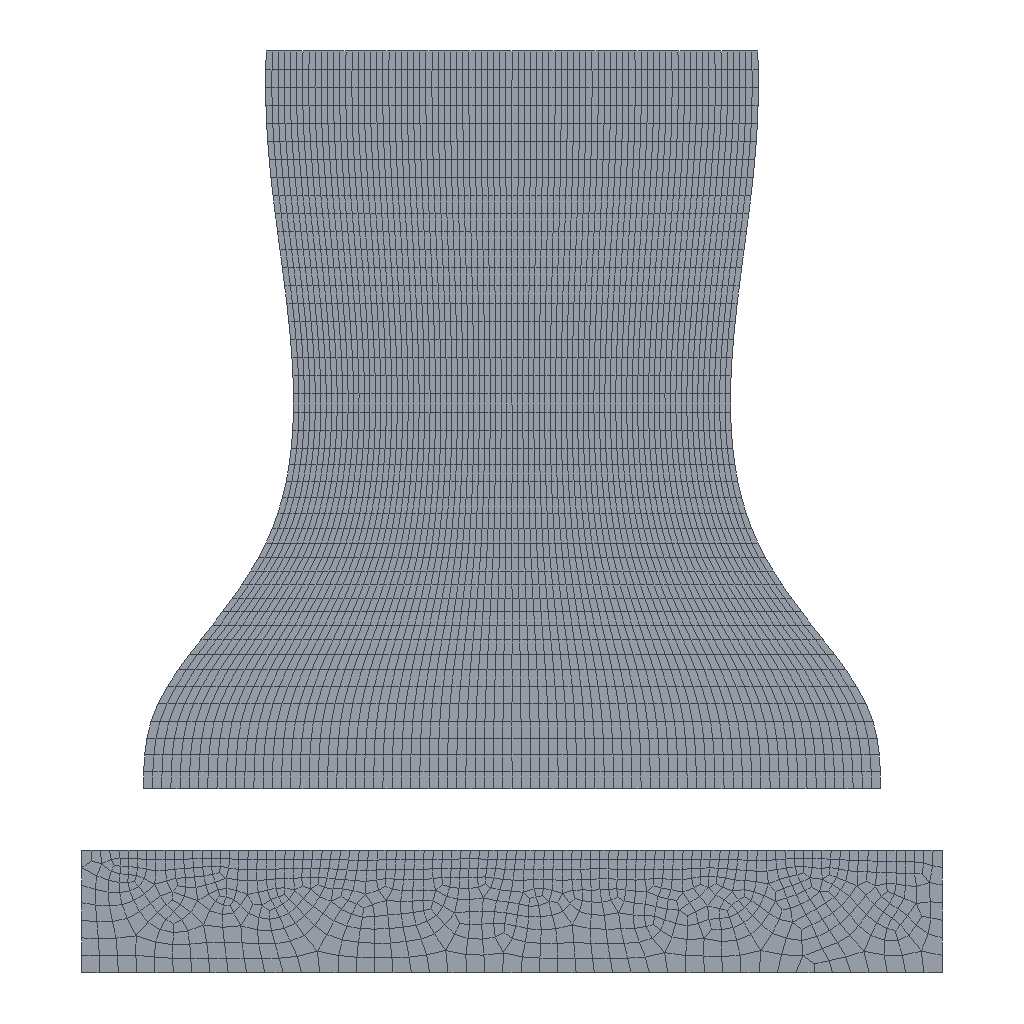Simulation study | abaqus
Set-up summary:
category,name,step,type,value,unit,region
solver,abaqus
solver,version,,,Abaqus/Standard 2020
units,not stated in the deck,,not stated
analysis,deck,,static,static
load_step,Step-1,Step-1,static
load_step,Step-3,Step-3,static
load_step,requested,,,2
mesh,nodes,,,4490
mesh,elements,,,4287
element_type,CPS4R,,plane,4287
load,load commands in deck,,count,2
bc,support commands in deck,,count,5
material,MIRROR,,in results
material,PDMS,,in results
material,SILICONRUBBER,,in results
material,TPU,,in results
material,TPU-COPY,,in results
material,TPU-COPY2,,in results
material,TPU-COPY3,,in results
material,TPU-COPY4,,in results
material,TPU-COPY5,,in results
check,setup vs results,,match,"per instance, exact: element labels, types and connectivity; labels of the nodes the elements use; coordinates of those nodes at SINGLE_PRECISION in 2 of 2 instance(s)"
Abaqus input file, long lists of numbers shortened:
*Heading
** Job name: Job-2 Model name: Model-1-Copy
** Generated by: Abaqus/CAE 2020
*Preprint, echo=NO, model=NO, history=NO, contact=NO
**
** PARTS
**
*Part, name=Mirror
*Node
      1,   137.021,           0.
      2,   131.064,           0.
** (843 more lines like these left out)
*Element, type=CPS4R
  1,  33,  31, 494,  72
  2,  72, 494, 455,  73
** (765 more lines like these left out)
*Nset, nset=_PickedSet3, internal, generate
   1,  845,    1
*Elset, elset=_PickedSet3, internal, generate
   1,  767,    1
*Elset, elset=_Surf-Mirror_S2, internal
  13,  19,  26,  33,  46,  60,  66,  72,  78,  84,  91,  95, 109, 115, 121, 127
 134, 141, 148, 154, 160, 164, 177, 183, 189, 195, 283, 344, 347, 349, 351, 353
** (2 more lines like these left out)
*Elset, elset=_Surf-Mirror_S4, internal
  40,  53, 102, 171, 284, 285, 287, 289, 290, 292, 293, 295, 296, 297, 299, 301
 303, 305, 307, 309, 310, 311, 313, 315, 317, 319, 321, 323, 325, 327, 329, 331
** (1 more lines like these left out)
*Elset, elset=_Surf-Mirror_S1, internal
 200, 383
*Elset, elset=_Surf-Mirror_S3, internal
 341,
*Surface, type=ELEMENT, name=Surf-Mirror
_Surf-Mirror_S2, S2
_Surf-Mirror_S4, S4
_Surf-Mirror_S1, S1
_Surf-Mirror_S3, S3
** Section: Section-mirror
*Solid Section, elset=_PickedSet3, material=Mirror
,
*End Part
**
*Part, name=mushroom
*Node
      1,  -35.915,   15.373
      2,   35.915,   15.373
** (3643 more lines like these left out)
*Element, type=CPS4R
   1,    1,   17,  723,  216
   2,   17,   18,  724,  723
** (3518 more lines like these left out)
*Nset, nset=FORCE
 3,
*Nset, nset=BOTTOM
  11,  12, 469, 470, 471, 472, 473, 474, 475, 476, 477, 478, 479, 480, 481, 482
 483, 484, 485, 486, 487, 488, 489, 490, 491, 492, 493, 494, 495, 496, 497, 498
** (4 more lines like these left out)
*Elset, elset=BOTTOM, generate
 2641,  2720,     1
*Nset, nset=Set-16
    1,    2,    3,    4,   17,   18,   19,   20,   21,   22,   23,   24,   25,   26,   27,   28
   29,   30,   31,   32,   33,   34,   35,   36,   37,   38,   39,   40,   41,   42,   43,   44
** (115 more lines like these left out)
*Elset, elset=Set-16, generate
    1,  1760,     1
*Nset, nset=Set-17
    9,   10,   11,   12,  387,  388,  389,  390,  391,  392,  393,  394,  395,  396,  397,  398
  399,  400,  401,  402,  403,  404,  405,  406,  407,  408,  409,  410,  411,  412,  413,  414
** (24 more lines like these left out)
*Elset, elset=Set-17, generate
 2401,  2720,     1
*Nset, nset=Set-18
    9,   10,   15,   16,  387,  388,  389,  390,  391,  392,  393,  394,  395,  396,  397,  398
  399,  400,  401,  402,  403,  404,  405,  406,  407,  408,  409,  410,  411,  412,  413,  414
** (19 more lines like these left out)
*Elset, elset=Set-18, generate
 3041,  3280,     1
*Nset, nset=Set-19
   13,   14,   15,   16,  554,  555,  556,  557,  558,  559,  560,  561,  562,  563,  564,  565
  566,  567,  568,  569,  570,  571,  572,  573,  574,  575,  576,  577,  578,  579,  580,  581
** (19 more lines like these left out)
*Elset, elset=Set-19, generate
 3281,  3520,     1
*Nset, nset=Set-20
    7,    8,   13,   14,  302,  303,  304,  305,  306,  307,  308,  309,  310,  311,  312,  313
  314,  315,  316,  317,  318,  319,  320,  321,  322,  323,  324,  325,  326,  327,  328,  329
** (24 more lines like these left out)
*Elset, elset=Set-20, generate
 2721,  3040,     1
*Nset, nset=Set-21
    5,    6,    7,    8,  220,  221,  222,  223,  224,  225,  226,  227,  228,  229,  230,  231
  232,  233,  234,  235,  236,  237,  238,  239,  240,  241,  242,  243,  244,  245,  246,  247
** (24 more lines like these left out)
*Elset, elset=Set-21, generate
 2081,  2400,     1
*Nset, nset=Set-22
    1,    2,    5,    6,   17,   18,   19,   20,   21,   22,   23,   24,   25,   26,   27,   28
   29,   30,   31,   32,   33,   34,   35,   36,   37,   38,   39,   40,   41,   42,   43,   44
** (24 more lines like these left out)
*Elset, elset=Set-22, generate
 1761,  2080,     1
*Elset, elset=_Surf-BOTTOM_S3, internal, generate
 2641,  2720,     1
*Surface, type=ELEMENT, name=Surf-BOTTOM
_Surf-BOTTOM_S3, S3
** Section: pdm
*Solid Section, elset=Set-16, material=PDMS
,
** Section: tpu6
*Solid Section, elset=Set-22, material=TPU-Copy5
,
** Section: tpu5
*Solid Section, elset=Set-21, material=TPU-Copy4
,
** Section: tpu1
*Solid Section, elset=Set-17, material=TPU
,
** Section: tpu4
*Solid Section, elset=Set-20, material=TPU-Copy3
,
** Section: tpu2
*Solid Section, elset=Set-18, material=TPU-Copy
,
** Section: tpu3
*Solid Section, elset=Set-19, material=TPU-Copy2
,
*End Part
**
**
** ASSEMBLY
**
*Assembly, name=Assembly
**
*Instance, name=Mirror-1, part=Mirror
        -70.,         -70.,           0.
*End Instance
**
*Instance, name=mushroom-1, part=mushroom
*End Instance
**
*Node
      1,         -70.,         -50.,           0.
*Node
      2,          70.,         -50.,           0.
*Nset, nset=Set-2, instance=Mirror-1
   1,   2,   3,   4,   5,   6,   7,   8,   9,  10,  11,  12,  13,  14,  15,  16
  17,  18,  19,  20,  21,  22,  23,  24,  25,  26,  27,  28,  29,  30,  31,  32
** (1 more lines like these left out)
*Elset, elset=Set-2, instance=Mirror-1
   1,   8,   9,  15,  21,  22,  28,  35,  36,  42,  48,  49,  55,  56,  62,  68
  69,  74,  80,  86,  87,  93,  97,  98, 104, 105, 117, 123, 129, 130, 136, 143
** (1 more lines like these left out)
*Nset, nset=Set-4, instance=mushroom-1
   3,   4, 117, 118, 119, 120, 121, 122, 123, 124, 125, 126, 127, 128, 129, 130
 131, 132, 133, 134, 135, 136, 137, 138, 139, 140, 141, 142, 143, 144, 145, 146
** (4 more lines like these left out)
*Elset, elset=Set-4, instance=mushroom-1, generate
 1681,  1760,     1
*End Assembly
*Amplitude, name=Amp-1
             0.,              0.,              1.,              1.
**
** MATERIALS
**
*Material, name=Mirror
*Density
 9.3e-07,
*Elastic
10000., 0.5
*Material, name=PDMS
*Density
 9.3e-07,
*Hyperelastic, neo hooke
 0.662, 0.255
*Material, name=SiliconRubber
*Density
 9.3e-07,
*Hyperelastic, mooney-rivlin
 0.111, 0.039, 0.001
*Material, name=TPU
*Density
 9.3e-07,
*Hyperelastic, ogden
 2.54, 3.29, 0.33
*Material, name=TPU-Copy
*Density
 9.3e-07,
*Hyperelastic, ogden
 1.54, 2.29, 0.33
*Material, name=TPU-Copy2
*Density
 9.3e-07,
*Hyperelastic, ogden
 0.54, 1.29, 0.33
*Material, name=TPU-Copy3
*Density
 9.3e-07,
*Hyperelastic, ogden
 0.24, 1.29, 0.33
*Material, name=TPU-Copy4
*Density
 9.3e-07,
*Hyperelastic, ogden
 0.14, 0.79, 0.33
*Material, name=TPU-Copy5
*Density
 9.3e-07,
*Hyperelastic, ogden
 0.14, 0.19, 0.33
**
** INTERACTION PROPERTIES
**
*Surface Interaction, name=INTPROP-1
1.,
*Friction, slip tolerance=0.005
0.,
*Surface Behavior, pressure-overclosure=HARD
*Surface Interaction, name=INTPROP-COH
1.,
*Cohesive Behavior, REPEATED CONTACTS, eligibility=CURRENT CONTACTS
 0.25, 0.25, 0.25
*Damage Initiation, criterion=MAXS
 0.05, 0.05, 0.05
*Damage Evolution, type=DISPLACEMENT, softening=EXPONENTIAL
 0.205,2.
*Damage Stabilization
0.01
**
** BOUNDARY CONDITIONS
**
** Name: BC-2 Type: 对称/反对称/完全固定
*Boundary
Set-2, ENCASTRE
**
** INTERACTIONS
**
** Interaction: Int-1
*Contact
*Contact Inclusions, ALL EXTERIOR
*Contact Property Assignment
 ,  , INTPROP-1
** ----------------------------------------------------------------
**
** STEP: Step-1
**
*Step, name=Step-1, nlgeom=YES
*Static, stabilize=0.0002, allsdtol=0.05, continue=NO
0.01, 1., 1e-05, 0.1
**
** BOUNDARY CONDITIONS
**
** Name: [REDACTED] : Displacement/rotation angle
*Boundary, amplitude=Amp-1
Set-4, 1, 1
Set-4, 2, 2, -22.9
Set-4, 6, 6
**
** OUTPUT REQUESTS
**
*Restart, write, frequency=0
**
** FIELD OUTPUT: F-Output-1
**
*Output, field
*Node Output
CF, RF, RM, RT, U, V
*Element Output, directions=YES
E, LE, MISES, MISESONLY, PE, PEEQ, PEMAG, S, SSAVG
*Contact Output
CDISP, CSTRESS
**
** HISTORY OUTPUT: H-Output-1
**
*Output, history, variable=PRESELECT
*End Step
** ----------------------------------------------------------------
**
** STEP: Step-3
**
*Step, name=Step-3, nlgeom=YES, inc=10000000
*Static, stabilize=0.0002, allsdtol=0.05, continue=NO
0.001, 1., 1e-10, 0.01
**
** BOUNDARY CONDITIONS
**
** Name: [REDACTED] : Displacement/rotation angle
*Boundary, amplitude=Amp-1
Set-4, 2, 2, 30.
**
** OUTPUT REQUESTS
**
*Restart, write, frequency=0
**
** FIELD OUTPUT: F-Output-1
**
*Output, field
*Node Output
CF, RF, RM, RT, U, V
*Element Output, directions=YES
E, LE, MISES, MISESONLY, PE, PEEQ, PEMAG, S, SSAVG
*Contact Output
CDISP, CSTRESS
**
** HISTORY OUTPUT: H-Output-1
**
*Output, history, variable=PRESELECT
*End Step
Results summary:
result,step,,completed,increments=16 time=1.0/1.0
result,step,,partial,increments=47 time=5.016131904295089e-06/1.0
result,analysis,,,static
result,last_loadstep,,,2
result,primary field,,,U
result,reaction total,,FX,-0.0,model units
result,reaction total,,FY,27.086,model units
result,reaction total,,FZ,0.0,model units